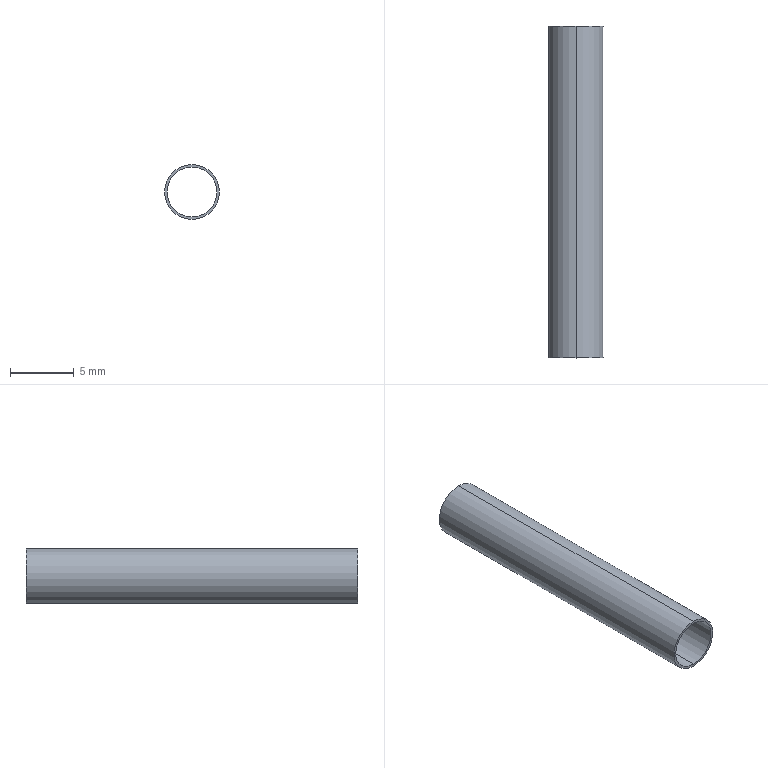Part | SolidWorks | features ExtruThin 1 | 1 solid | 6 faces | box 4.3 x 26 x 4.3 mm | volume 66.979 mm3 | cylinder 4 | plane 2 | commonest cylinder face diameters 3.9 x2 4.3 x2
STEP:
#1=CARTESIAN_POINT('',(0.,26.,-1.95));
#2=VERTEX_POINT('',#1);
#3=CARTESIAN_POINT('',(0.,26.,1.95));
#4=VERTEX_POINT('',#3);
#5=CARTESIAN_POINT('',(0.,26.,0.));
#6=DIRECTION('',(0.,1.,0.));
#7=DIRECTION('',(1.,0.,0.));
#8=AXIS2_PLACEMENT_3D('',#5,#6,#7);
#9=CIRCLE('',#8,1.95);
#10=EDGE_CURVE('',#2,#4,#9,.T.);
#11=ORIENTED_EDGE('',*,*,#10,.T.);
#12=CARTESIAN_POINT('',(0.,0.,1.95));
#13=VERTEX_POINT('',#12);
#14=CARTESIAN_POINT('',(0.,26.,1.95));
#15=DIRECTION('',(0.,-1.,0.));
#16=VECTOR('',#15,1000.);
#17=LINE('',#14,#16);
#18=EDGE_CURVE('',#4,#13,#17,.T.);
#19=ORIENTED_EDGE('',*,*,#18,.T.);
#20=CARTESIAN_POINT('',(0.,0.,-1.95));
#21=VERTEX_POINT('',#20);
#22=CARTESIAN_POINT('',(0.,0.,0.));
#23=DIRECTION('',(0.,1.,0.));
#24=DIRECTION('',(1.,0.,0.));
#25=AXIS2_PLACEMENT_3D('',#22,#23,#24);
#26=CIRCLE('',#25,1.95);
#27=EDGE_CURVE('',#21,#13,#26,.T.);
#28=ORIENTED_EDGE('',*,*,#27,.F.);
#29=CARTESIAN_POINT('',(0.,26.,-1.95));
#30=DIRECTION('',(0.,-1.,0.));
#31=VECTOR('',#30,1000.);
#32=LINE('',#29,#31);
#33=EDGE_CURVE('',#2,#21,#32,.T.);
#34=ORIENTED_EDGE('',*,*,#33,.F.);
#35=EDGE_LOOP('',(#11,#19,#28,#34));
#36=FACE_OUTER_BOUND('',#35,.T.);
#37=CARTESIAN_POINT('',(0.,26.,0.));
#38=DIRECTION('',(0.,-1.,0.));
#39=DIRECTION('',(0.,0.,-1.));
#40=AXIS2_PLACEMENT_3D('',#37,#38,#39);
#41=CYLINDRICAL_SURFACE('',#40,1.95);
#42=ADVANCED_FACE('',(#36),#41,.F.);
#43=CARTESIAN_POINT('',(0.,26.,2.15));
#44=VERTEX_POINT('',#43);
#45=CARTESIAN_POINT('',(0.,26.,-2.15));
#46=VERTEX_POINT('',#45);
#47=CARTESIAN_POINT('',(0.,26.,0.));
#48=DIRECTION('',(0.,1.,0.));
#49=DIRECTION('',(0.,0.,1.));
#50=AXIS2_PLACEMENT_3D('',#47,#48,#49);
#51=CIRCLE('',#50,2.15);
#52=EDGE_CURVE('',#44,#46,#51,.T.);
#53=ORIENTED_EDGE('',*,*,#52,.F.);
#54=CARTESIAN_POINT('',(0.,0.,2.15));
#55=VERTEX_POINT('',#54);
#56=CARTESIAN_POINT('',(0.,26.,2.15));
#57=DIRECTION('',(0.,-1.,0.));
#58=VECTOR('',#57,1000.);
#59=LINE('',#56,#58);
#60=EDGE_CURVE('',#44,#55,#59,.T.);
#61=ORIENTED_EDGE('',*,*,#60,.T.);
#62=CARTESIAN_POINT('',(0.,0.,-2.15));
#63=VERTEX_POINT('',#62);
#64=CARTESIAN_POINT('',(0.,0.,0.));
#65=DIRECTION('',(0.,1.,0.));
#66=DIRECTION('',(0.,0.,1.));
#67=AXIS2_PLACEMENT_3D('',#64,#65,#66);
#68=CIRCLE('',#67,2.15);
#69=EDGE_CURVE('',#55,#63,#68,.T.);
#70=ORIENTED_EDGE('',*,*,#69,.T.);
#71=CARTESIAN_POINT('',(0.,26.,-2.15));
#72=DIRECTION('',(0.,-1.,0.));
#73=VECTOR('',#72,1000.);
#74=LINE('',#71,#73);
#75=EDGE_CURVE('',#46,#63,#74,.T.);
#76=ORIENTED_EDGE('',*,*,#75,.F.);
#77=EDGE_LOOP('',(#53,#61,#70,#76));
#78=FACE_OUTER_BOUND('',#77,.T.);
#79=CARTESIAN_POINT('',(0.,26.,0.));
#80=DIRECTION('',(0.,-1.,0.));
#81=DIRECTION('',(0.,0.,-1.));
#82=AXIS2_PLACEMENT_3D('',#79,#80,#81);
#83=CYLINDRICAL_SURFACE('',#82,2.15);
#84=ADVANCED_FACE('',(#78),#83,.T.);
#85=CARTESIAN_POINT('',(0.,26.,0.));
#86=DIRECTION('',(0.,1.,0.));
#87=DIRECTION('',(0.,0.,1.));
#88=AXIS2_PLACEMENT_3D('',#85,#86,#87);
#89=CIRCLE('',#88,2.15);
#90=EDGE_CURVE('',#46,#44,#89,.T.);
#91=ORIENTED_EDGE('',*,*,#90,.T.);
#92=ORIENTED_EDGE('',*,*,#52,.T.);
#93=EDGE_LOOP('',(#91,#92));
#94=FACE_OUTER_BOUND('',#93,.T.);
#95=ORIENTED_EDGE('',*,*,#10,.F.);
#96=CARTESIAN_POINT('',(0.,26.,0.));
#97=DIRECTION('',(0.,1.,0.));
#98=DIRECTION('',(1.,0.,0.));
#99=AXIS2_PLACEMENT_3D('',#96,#97,#98);
#100=CIRCLE('',#99,1.95);
#101=EDGE_CURVE('',#4,#2,#100,.T.);
#102=ORIENTED_EDGE('',*,*,#101,.F.);
#103=EDGE_LOOP('',(#95,#102));
#104=FACE_BOUND('',#103,.T.);
#105=CARTESIAN_POINT('',(0.,26.,0.));
#106=DIRECTION('',(0.,1.,0.));
#107=DIRECTION('',(0.,0.,1.));
#108=AXIS2_PLACEMENT_3D('',#105,#106,#107);
#109=PLANE('',#108);
#110=ADVANCED_FACE('',(#94,#104),#109,.T.);
#111=CARTESIAN_POINT('',(0.,0.,0.));
#112=DIRECTION('',(0.,1.,0.));
#113=DIRECTION('',(0.,0.,1.));
#114=AXIS2_PLACEMENT_3D('',#111,#112,#113);
#115=CIRCLE('',#114,2.15);
#116=EDGE_CURVE('',#63,#55,#115,.T.);
#117=ORIENTED_EDGE('',*,*,#116,.F.);
#118=ORIENTED_EDGE('',*,*,#69,.F.);
#119=EDGE_LOOP('',(#117,#118));
#120=FACE_OUTER_BOUND('',#119,.T.);
#121=ORIENTED_EDGE('',*,*,#27,.T.);
#122=CARTESIAN_POINT('',(0.,0.,0.));
#123=DIRECTION('',(0.,1.,0.));
#124=DIRECTION('',(1.,0.,0.));
#125=AXIS2_PLACEMENT_3D('',#122,#123,#124);
#126=CIRCLE('',#125,1.95);
#127=EDGE_CURVE('',#13,#21,#126,.T.);
#128=ORIENTED_EDGE('',*,*,#127,.T.);
#129=EDGE_LOOP('',(#121,#128));
#130=FACE_BOUND('',#129,.T.);
#131=CARTESIAN_POINT('',(0.,0.,0.));
#132=DIRECTION('',(0.,1.,0.));
#133=DIRECTION('',(0.,0.,1.));
#134=AXIS2_PLACEMENT_3D('',#131,#132,#133);
#135=PLANE('',#134);
#136=ADVANCED_FACE('',(#120,#130),#135,.F.);
#137=ORIENTED_EDGE('',*,*,#60,.F.);
#138=ORIENTED_EDGE('',*,*,#90,.F.);
#139=ORIENTED_EDGE('',*,*,#75,.T.);
#140=ORIENTED_EDGE('',*,*,#116,.T.);
#141=EDGE_LOOP('',(#137,#138,#139,#140));
#142=FACE_OUTER_BOUND('',#141,.T.);
#143=CARTESIAN_POINT('',(0.,26.,0.));
#144=DIRECTION('',(0.,-1.,0.));
#145=DIRECTION('',(0.,0.,-1.));
#146=AXIS2_PLACEMENT_3D('',#143,#144,#145);
#147=CYLINDRICAL_SURFACE('',#146,2.15);
#148=ADVANCED_FACE('',(#142),#147,.T.);
#149=ORIENTED_EDGE('',*,*,#18,.F.);
#150=ORIENTED_EDGE('',*,*,#101,.T.);
#151=ORIENTED_EDGE('',*,*,#33,.T.);
#152=ORIENTED_EDGE('',*,*,#127,.F.);
#153=EDGE_LOOP('',(#149,#150,#151,#152));
#154=FACE_OUTER_BOUND('',#153,.T.);
#155=CARTESIAN_POINT('',(0.,26.,0.));
#156=DIRECTION('',(0.,-1.,0.));
#157=DIRECTION('',(0.,0.,-1.));
#158=AXIS2_PLACEMENT_3D('',#155,#156,#157);
#159=CYLINDRICAL_SURFACE('',#158,1.95);
#160=ADVANCED_FACE('',(#154),#159,.F.);
#161=CLOSED_SHELL('',(#42,#84,#110,#136,#148,#160));
#162=MANIFOLD_SOLID_BREP('',#161);
#163=CARTESIAN_POINT('',(0.,0.,0.));
#164=DIRECTION('',(0.,0.,1.));
#165=DIRECTION('',(1.,0.,0.));
#166=AXIS2_PLACEMENT_3D('',#163,#164,#165);
#167=(LENGTH_UNIT()NAMED_UNIT(*)SI_UNIT(.MILLI.,.METRE.));
#168=UNCERTAINTY_MEASURE_WITH_UNIT(LENGTH_MEASURE(0.00001),#167,'','');
#169=(NAMED_UNIT(*)PLANE_ANGLE_UNIT()SI_UNIT($,.RADIAN.));
#170=(NAMED_UNIT(*)SI_UNIT($,.STERADIAN.)SOLID_ANGLE_UNIT());
#171=(GEOMETRIC_REPRESENTATION_CONTEXT(3)GLOBAL_UNCERTAINTY_ASSIGNED_CONTEXT((#168))GLOBAL_UNIT_ASSIGNED_CONTEXT((#167,#169,#170))REPRESENTATION_CONTEXT('',''));
#172=ADVANCED_BREP_SHAPE_REPRESENTATION('',(#162,#166),#171);